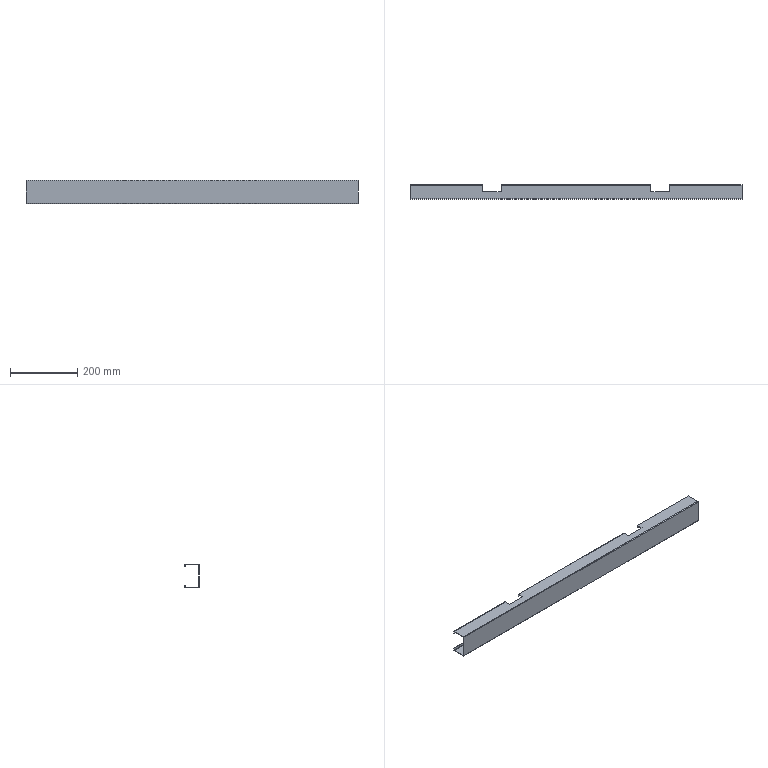Part | 1 solid | 86 faces | box 985 x 42 x 70 mm | volume 231133 mm3 | plane 70 | cylinder 16 | commonest cylinder face diameters 0.4 x8 3.4 x8